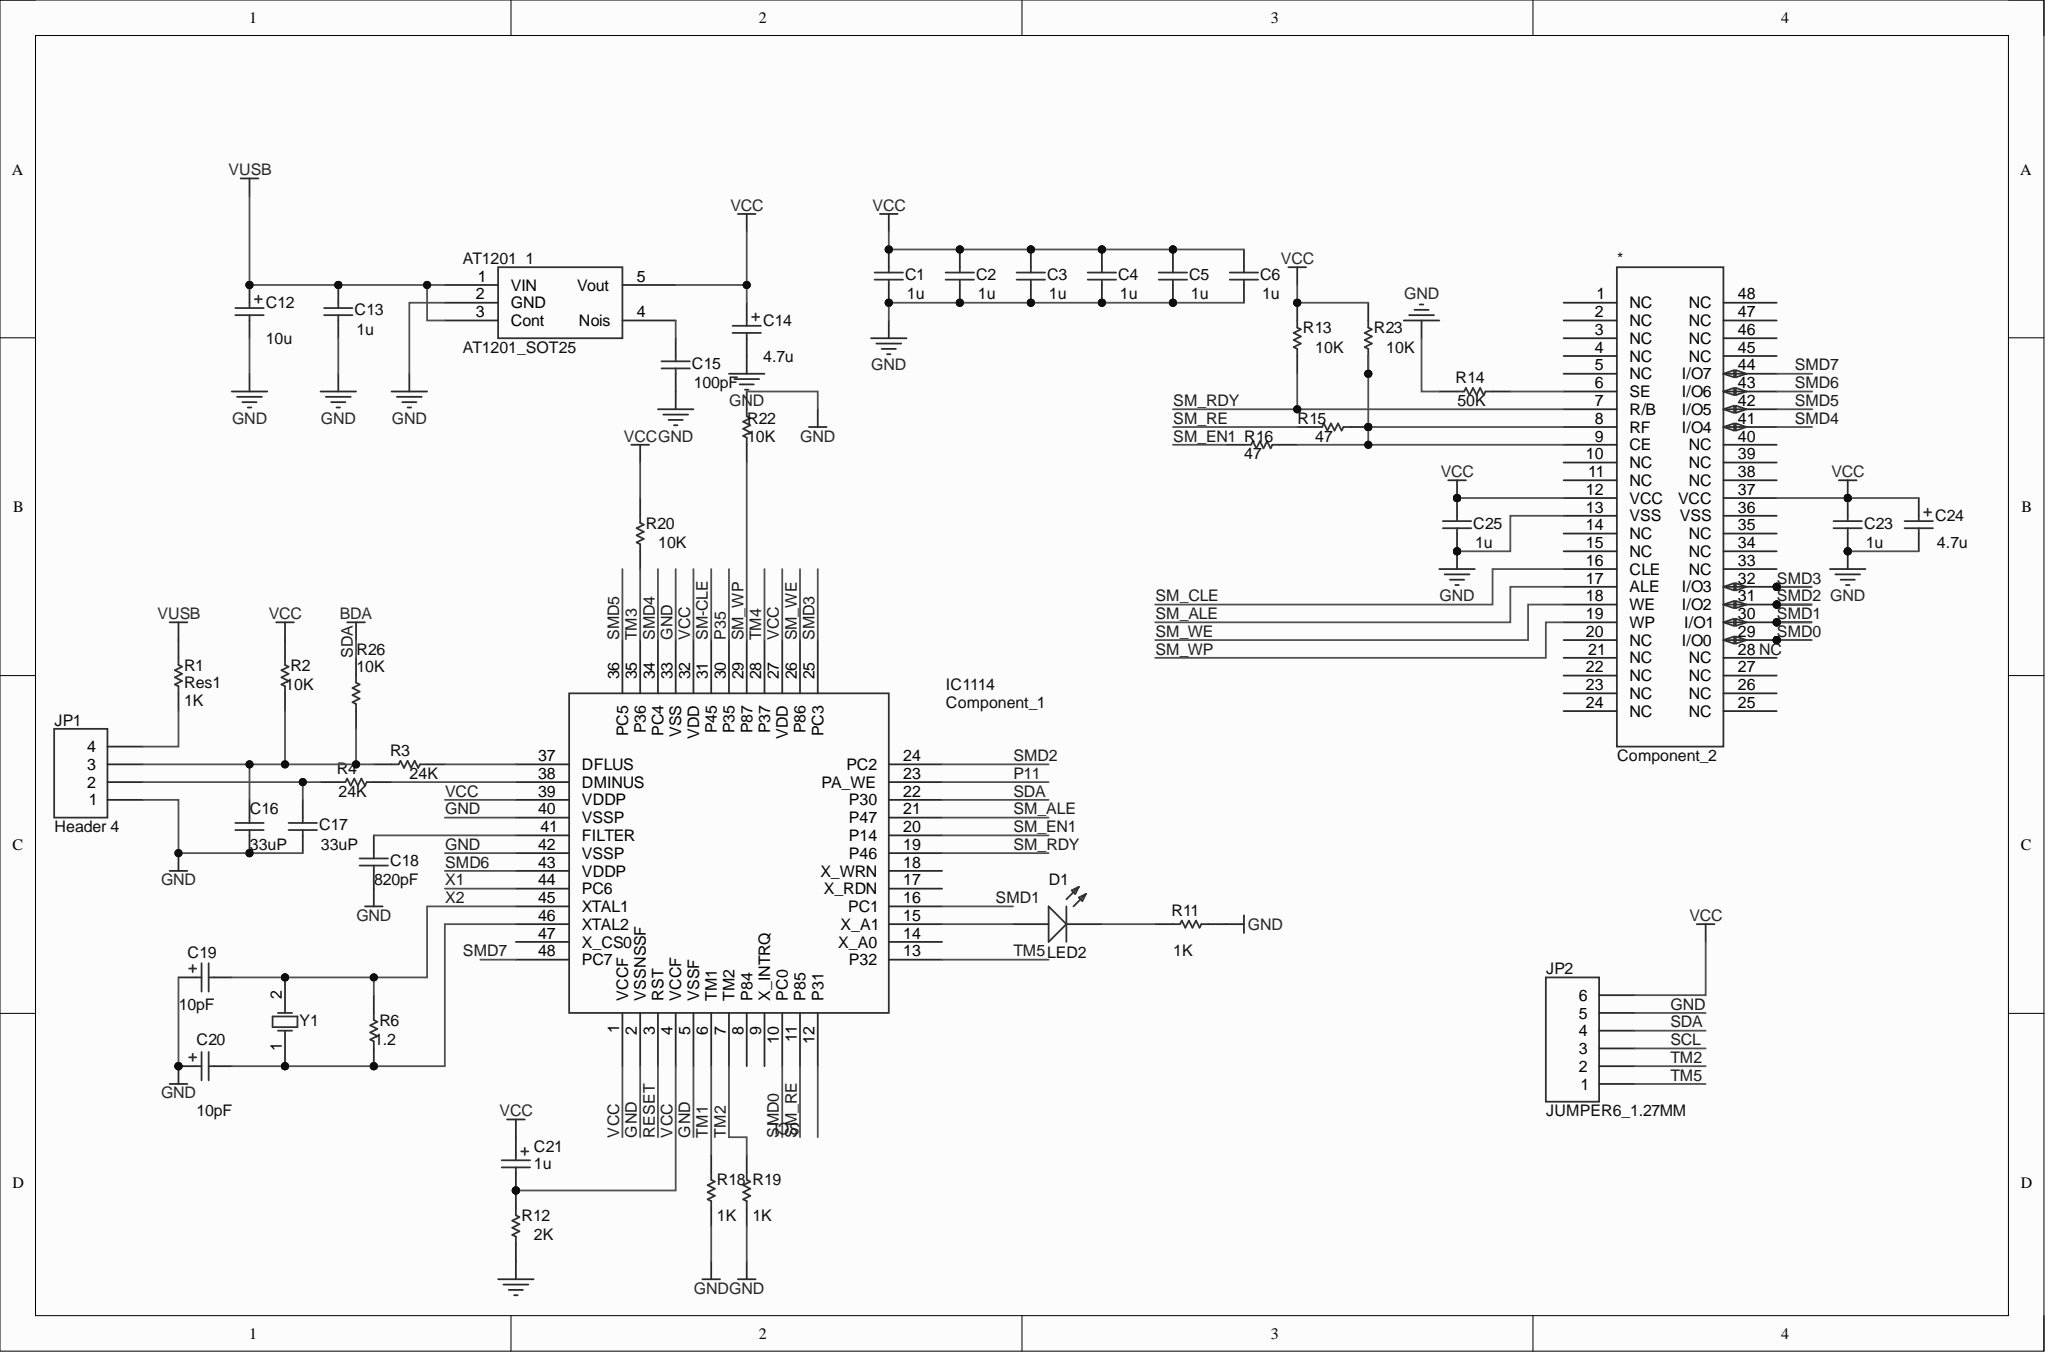Circuit board | Altium Designer | 43 parts | 34 nets
Bill of materials:
Comment,Description,Designator,Footprint,LibRef,Quantity
"Component_2","","","DIP48","Component_2","1"
"AT1201_SOT25","","AT1201  1","SOP6","AT1201_SOT25","1"
"","Capacitor","C1, C2, C3, C4, C5, C6, C13, C15, C16, C17, C18, C23, C25","RAD-0.3","C1, C2, C3, C4, C5, C6, C13, C15, C16, C17, C18, C23, C25","13"
"","Polarized Capacitor (Axial)","C12, C14, C19, C20, C21, C24","POLAR0.8","C12, C14, C19, C20, C21, C24","6"
"LED2","Typical RED, GREEN, YELLOW, AMBER GaAs LED","D1","3.2X1.6X1.1","LED2","1"
"Component_1","","IC1114","Quad48","Component_1","1"
"Header 4","Header, 4-Pin","JP1","HDR1X4","Header 4","1"
"JUMPER6_1.27MM","Header, 6-Pin","JP2","HDR1X6","JUMPER6_1.27MM","1"
"Res1","Resistor","R1","AXIAL-0.3","Res1","1"
"","Resistor","R2, R3, R4, R6, R11, R12, R13, R14, R15, R16, R18, R19, R20, R22, R23, R26","AXIAL-0.3","R2, R3, R4, R6, R11, R12, R13, R14, R15, R16, R18, R19, R20, R22, R23, R26","16"
"","Crystal Oscillator","Y1","R38","Y1","1"
Netlist (Protel format):
[
*
DIP48
Component_2



]
[
AT1201  1
SOP6
AT1201_SOT25



]
[
C1
RAD-0.3




]
[
C2
RAD-0.3




]
[
C3
RAD-0.3




]
[
C4
RAD-0.3




]
[
C5
RAD-0.3




]
[
C6
RAD-0.3




]
[
C12
POLAR0.8




]
[
C13
RAD-0.3




]
[
C14
POLAR0.8




]
[
C15
RAD-0.3




]
[
C16
RAD-0.3




]
[
C17
RAD-0.3




]
[
C18
RAD-0.3




]
[
C19
POLAR0.8




]
[
C20
POLAR0.8




]
[
C21
POLAR0.8




]
[
C23
RAD-0.3




]
[
C24
POLAR0.8




]
[
C25
RAD-0.3




]
[
D1
3.2X1.6X1.1
LED2



]
[
IC1114
Quad48
Component_1



]
[
JP1
HDR1X4
Header 4



]
[
JP2
HDR1X6
JUMPER6_1.27MM



]
[
R1
AXIAL-0.3
Res1



]
[
R2
AXIAL-0.3




]
[
R3
AXIAL-0.3




]
[
R4
AXIAL-0.3




]
[
R6
AXIAL-0.3




]
[
R11
AXIAL-0.3




]
[
R12
AXIAL-0.3




]
[
R13
AXIAL-0.3




]
[
R14
AXIAL-0.3




]
[
R15
AXIAL-0.3




]
[
R16
AXIAL-0.3




]
[
R18
AXIAL-0.3




]
[
R19
AXIAL-0.3




]
[
R20
AXIAL-0.3




]
[
R22
AXIAL-0.3




]
[
R23
AXIAL-0.3




]
[
R26
AXIAL-0.3




]
[
Y1
R38




]
(
X2
C19-2
IC1114-45
R6-2
Y1-2
)
(
VUSB
AT1201  1-1
AT1201  1-3
C12-1
C13-2
R1-2
)
(
VCC
*-12
*-37
AT1201  1-5
C1-2
C2-2
C3-2
C4-2
C5-2
C6-2
C14-1
C21-1
C21-2
C23-2
C24-1
C25-2
IC1114-1
IC1114-4
IC1114-27
IC1114-32
IC1114-39
JP2-6
R2-2
R12-2
R13-2
R20-2
R23-2
)
(
TM5
IC1114-13
JP2-1
)
(
TM3
IC1114-35
R20-1
)
(
TM2
IC1114-7
JP2-2
R19-2
)
(
TM1
IC1114-6
R18-2
)
(
SMD6
*-43
IC1114-43
)
(
SMD5
*-42
IC1114-36
)
(
SMD4
*-41
IC1114-34
)
(
SMD3
*-32
IC1114-25
)
(
SMD2
*-31
IC1114-24
)
(
SMD1
*-30
IC1114-16
)
(
SMD0
*-29
IC1114-10
)
(
SM_WP
*-19
IC1114-29
R22-1
)
(
SM_WE
*-18
IC1114-26
)
(
SM_RDY
*-7
IC1114-19
R13-1
)
(
SM_EN1
IC1114-20
R16-1
)
(
SM_ALE
*-17
IC1114-21
)
(
SDA
IC1114-22
JP2-4
R26-2
)
(
SCL
IC1114-11
JP2-3
R15-1
)
(
NetJP1_4
JP1-4
R1-1
)
(
NetIC1114_38
IC1114-38
R4-2
)
(
NetIC1114_37
IC1114-37
R3-2
)
(
NetD1_2
D1-2
R11-1
)
(
NetD1_1
D1-1
IC1114-15
)
(
NetC20_2
C20-2
IC1114-46
R6-1
Y1-1
)
(
NetC18_2
C18-2
IC1114-41
)
(
NetC17_1
C17-1
JP1-2
R4-1
)
(
NetC16_2
C16-2
JP1-3
R2-1
R3-1
R26-1
)
(
NetAT1201  1_4
AT1201  1-4
C15-2
)
(
Net*_8
*-8
*-9
R15-2
R16-2
R23-1
)
(
Net*_6
*-6
R14-1
)
(
GND
*-13
AT1201  1-2
C1-1
C2-1
C3-1
C4-1
C5-1
C6-1
C12-2
C13-1
C14-2
C15-1
C16-1
C17-2
C18-1
C19-1
C20-1
C23-1
C24-2
C25-1
IC1114-2
IC1114-5
IC1114-33
IC1114-40
IC1114-42
JP1-1
JP2-5
R11-2
R12-1
R14-2
R18-1
R19-1
R22-2
)